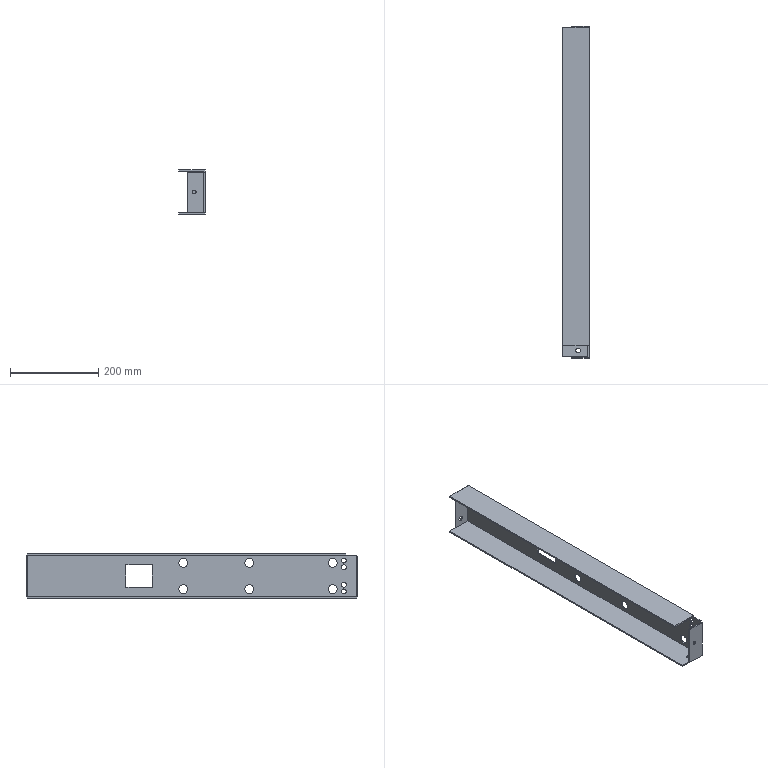Part | SolidWorks | features BaseBody 1 | 1 solid | 56 faces | box 60 x 754 x 100 mm | volume 481088 mm3 | cylinder 28 | plane 28 | commonest cylinder face diameters 11 x12 20 x12 8.5 x2 10.6 x2